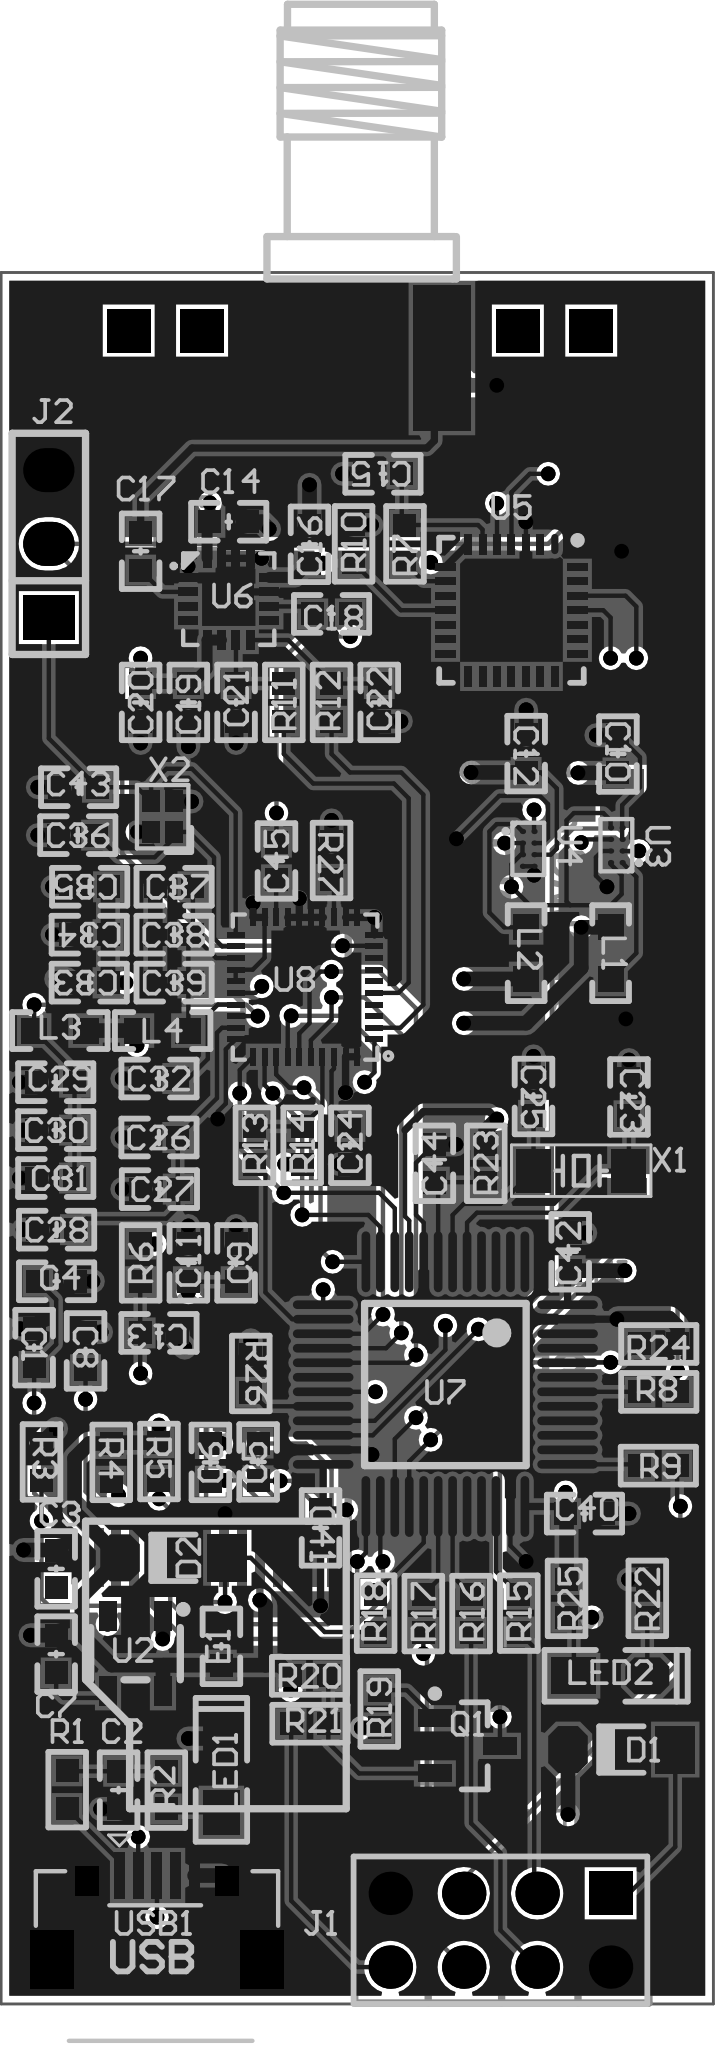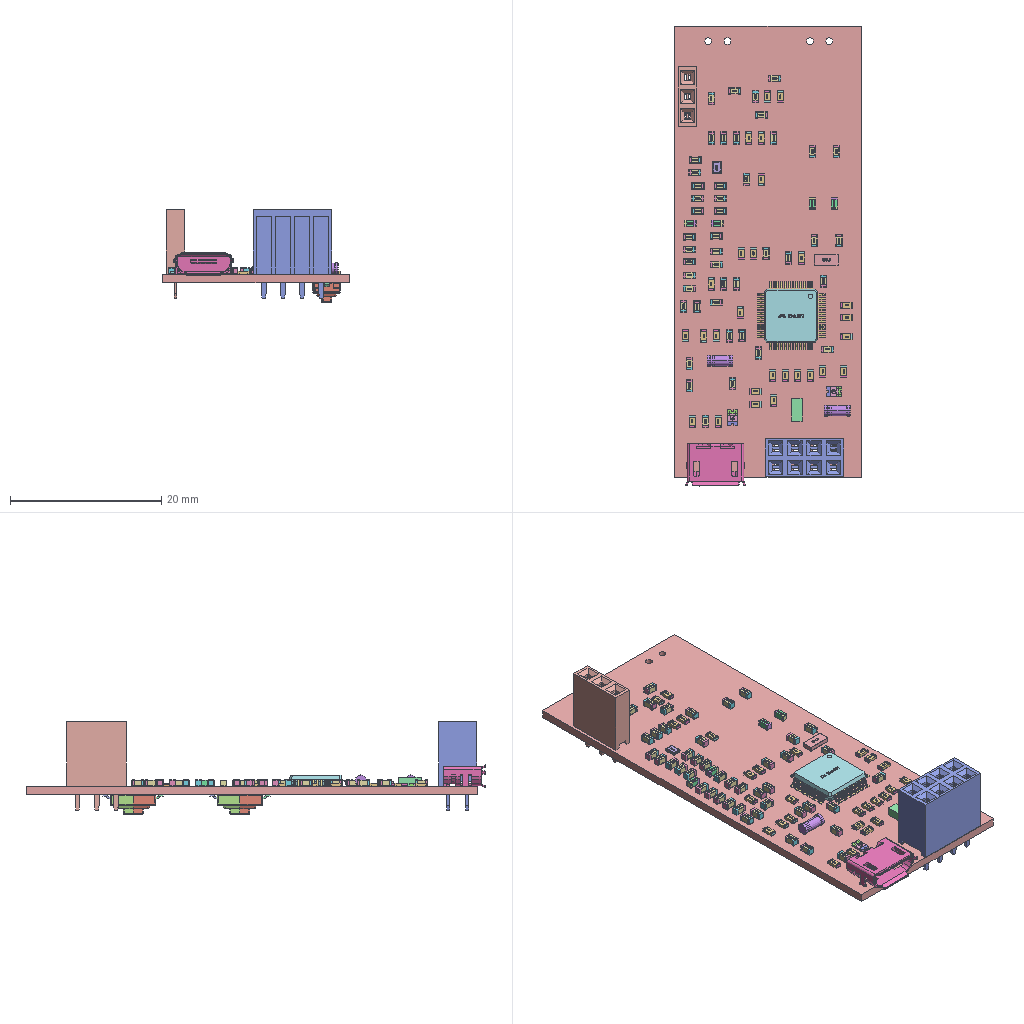Circuit board layout | Altium Designer | box 24.6 x 60.8 x 12.2 mm
Layer stack:
# Altium Designer layer stack of  (unit mm; dielectric type: 0 none, 1 core, 2 prepreg, 3 surface material)
index,name,kind,layer,copper_thickness_mm,dielectric_type,dielectric_thickness_mm,dielectric_material,dielectric_constant
0,Top Paste,other,,,,,,
1,Top Overlay,other,,,,,,
2,Top Solder,dielectric,,,3,0.0102,Solder Resist,3.5
3,Top Layer,copper,Top Layer,0.0356,,,,
4,Dielectric1,dielectric,,,1,0.32,FR-4,4.8
5,SIGN,copper,SIGN,0.0356,,,,
6,Dielectric3,dielectric,,,1,0.32,FR-4,4.8
7,VCC,copper,VCC,0.0356,,,,
8,Dielectric2,dielectric,,,2,0.32,FR-4,4.8
9,Bottom Layer,copper,Bottom Layer,0.0356,,,,
10,Bottom Solder,dielectric,,,3,0.0102,Solder Resist,3.5
11,Bottom Overlay,other,,,,,,
12,Bottom Paste,other,,,,,,
# drill layer pairs: low layer,high layer
drill_pair,Top Layer,Bottom Layer
Part placement:
Designator,Comment,Layer,Footprint,Center-X(mm),Center-Y(mm),Rotation
U1,0.91-OLED,BottomLayer,OLED0.91,4.987,15.367,270
X2,38.4MHZ,TopLayer,OSC_1612-4P,3.175,40.894,90
X1,16MHz,TopLayer,OSC_3215-2P,17.653,28.702,360
USB1,USB-5P,TopLayer,USB-MICRO_A,2.979,2.974,0
U8,DW3210,TopLayer,DW3210,8.101,35.025,180
U7,STM32F103C8T6,TopLayer,LQFP48_7X7,12.954,21.349,180
U6,SW8112Q,TopLayer,QFN-16_L3.0-W3.0-P0.50-BL-EP1.7,5.461,48.387,270
U5,CP2102,TopLayer,CP2102,15.24,48.006,270
U4,TPS62743YFPR,TopLayer,DSBGA-8_L1.6-W0.9-R2-C4-P0.40-BL,15.821,39.786,270
U3,TPS62743YFPR,TopLayer,DSBGA-8_L1.6-W0.9-R2-C4-P0.40-BL,18.869,39.913,90
U2,TPS736,TopLayer,SOT-23-5_L3.0-W1.7-P0.95-LS2.8-BR,2.236,12.065,90
SW2,3x6x5,BottomLayer,TSW_SMD-3*6*2.5,19.06,45.495,270
SW1,3x6x5,BottomLayer,TSW_SMD-3*6*2.5,19.187,31.398,270
R27,49R9,TopLayer,R_0603_L,9.017,39.385,270
R26,10K,TopLayer,R_0603_L,6.223,21.717,90
R25,10K,TopLayer,R_0603_L,17.145,13.97,90
R24,10K,TopLayer,R_0603_L,20.335,22.733,360
R23,1K,TopLayer,R_0603_L,14.351,28.956,90
R22,470R,TopLayer,R_0603_L,19.939,13.97,90
R21,1K,TopLayer,R_0603_L,8.27,9.652,360
R20,1K,TopLayer,R_0603_L,8.255,11.303,360
R19,1K,TopLayer,R_0603_L,10.668,10.16,90
R18,22R,TopLayer,R_0603_L,10.541,13.462,90
R17,22R,TopLayer,R_0603_L,12.192,13.447,90
R16,22R,TopLayer,R_0603_L,13.843,13.447,90
R15,22R,TopLayer,R_0603_L,15.494,13.462,90
R14,DNF,TopLayer,R_0603_L,8.001,29.576,90
R13,100R,TopLayer,R_0603_L,6.35,29.576,90
R12,0R,TopLayer,R_0603_L,9.017,44.831,90
R11,0R,TopLayer,R_0603_L,7.366,44.831,90
R10,10K,TopLayer,R_0603_L,9.779,50.292,270
R9,22R,TopLayer,R_0603_L,20.32,18.542,0
R8,0R,TopLayer,R_0603_L,20.335,21.082,0
R7,4.7K,TopLayer,R_0603_L,11.557,50.292,90
R6,4.7K,TopLayer,R_0603_L,2.413,25.527,90
R5,4.7K,TopLayer,R_0603_L,3.048,18.684,270
R4,4.7K,TopLayer,R_0603_L,1.397,18.654,270
R3,4.7K,TopLayer,R_0603_L,-1.016,18.669,270
R2,470R,TopLayer,R_0603_L,3.302,7.366,90
R1,B5R,TopLayer,R_0603_L,-0.127,7.381,90
Q1,S9012,TopLayer,SOT-23B_N,13.716,8.89,360
LED2,Red,TopLayer,LED_0805G,18.669,11.303,360
LED1,Red,TopLayer,LED_0805G,5.207,7.874,90
L4,600R,TopLayer,L_0603,3.175,33.528,180
L3,600R,TopLayer,L_0603,-0.381,33.528,360
L2,Inductor Iron,TopLayer,L_0603,15.748,36.195,270
L1,Inductor Iron,TopLayer,L_0603,18.669,36.195,90
J2,Female HDR1X3,TopLayer,Fe-HDR1X3/2.54-S,-0.762,50.292,180
J1,Female HDR2X4,TopLayer,Fe-HDR2X4/2.54-S,14.859,2.54,180
E1,22uF/6.3V,TopLayer,C_0603_L,5.207,12.319,90
D2,1N4148,TopLayer,MINI_MELF_(LL34),3.556,15.367,180
D1,SS34,TopLayer,MINI_MELF_(LL34),19.05,8.763,180
C45,2pF,TopLayer,C_0603_L,7.112,39.37,90
C44,100nF,TopLayer,C_0603_L,12.573,28.956,90
C43,8pF,TopLayer,C_0603_L,0.269,41.91,360
C42,100nF,TopLayer,C_0603_L,17.272,25.908,90
C41,100nF,TopLayer,C_0603_L,8.636,16.398,270
C40,100nF,TopLayer,C_0603_L,17.765,16.891,360
C39,10uF,TopLayer,C_0603_L,3.571,35.179,360
C38,100nF,TopLayer,C_0603_L,3.571,36.83,360
C37,4.7nF,TopLayer,C_0603_L,3.571,38.481,360
C36,8pF,TopLayer,C_0603_L,0.239,40.259,360
C35,10uF,TopLayer,C_0603_L,0.65,38.481,180
C34,100nF,TopLayer,C_0603_L,0.6351,36.83,180
C33,4.7nF,TopLayer,C_0603_L,0.6351,35.179,180
C32,220nF,TopLayer,C_0603_L,3.048,31.877,180
C31,10uF,TopLayer,C_0603_L,-0.523,28.448,360
C30,100nF,TopLayer,C_0603_L,-0.523,30.099,360
C29,4.7nF,TopLayer,C_0603_L,-0.523,31.75,360
C28,22uF,TopLayer,C_0603_L,-0.493,26.67,360
C27,100nF,TopLayer,C_0603_L,3.063,28.067,360
C26,2pF,TopLayer,C_0603_L,3.048,29.845,360
C25,20pF,TopLayer,C_0603_L,16.002,31.257,270
C24,100nF,TopLayer,C_0603_L,9.652,29.576,90
C23,20pF,TopLayer,C_0603_L,19.304,31.242,270
C22,1nF,TopLayer,C_0603_L,10.668,44.831,270
C21,1nF,TopLayer,C_0603_L,5.715,44.831,270
C20,1nF,TopLayer,C_0603_L,2.413,44.831,270
C19,1nF,TopLayer,C_0603_L,4.064,44.831,270
C18,100pF,TopLayer,C_0603_L,9.017,47.879,180
C17,100pF,TopLayer,C_0603_L,2.413,50.038,90
C16,1nF,TopLayer,C_0603_L,8.255,50.277,90
C15,4.7uF,TopLayer,C_0603_L,10.795,52.705,360
C14,1nF,TopLayer,C_0603_L,5.461,51.054,360
C13,4.7uF,TopLayer,C_0603_L,3.048,23.114,180
C12,10uF,TopLayer,C_0603_L,15.748,43.068,270
C11,4.7uF,TopLayer,C_0603_L,4.064,25.527,90
C10,10uF,TopLayer,C_0603_L,18.923,43.053,270
C9,100nF,TopLayer,C_0603_L,5.715,25.527,90
C8,2.2uF,TopLayer,C_0603_L,0.508,22.494,270
C7,100nF,TopLayer,C_0603_L,-0.508,12.05,270
C6,1uF,TopLayer,C_0603_L,4.826,18.654,90
C5,1uF,TopLayer,C_0603_L,6.477,18.669,90
C4,4.7uF,TopLayer,C_0603_L,-0.493,24.892,180
C3,10uF,TopLayer,C_0603_L,-0.5081,14.986,270
C2,100nF,TopLayer,C_0603_L,1.651,7.366,90
C1,100nF,TopLayer,C_0603_L,-1.27,22.606,270
ANT1,Partron,TopLayer,天线座5p,10.033,56.685,90
Pad and via stacks:
# Altium Designer via and pad stacks of  (unit mm). Each distinct definition once, with the count of objects using it.
# via: kind,start_layer,end_layer,hole_mm,diameter_mm,mode(0 simple;1 top-mid-bottom;2 full stack),diameter_per_layer,count,example_net
# pad: kind,layer,hole_mm,hole_type(0 round;1 square;2 slot),plating,top_size,top_shape(1 round;2 rect;3 octagon;9 rounded rect),mid_size,bottom_size,mode,footprint,size_per_layer,count,example
pad,Multi-Layer,0.5,2,plated,1.5x2,2,1.5x2,1.5x2,0,USB-MICRO_A,,2,USB1.5
pad,Multi-Layer,0.5,0,plated,0.8x1,2,0.8x1,0.8x1,0,USB-MICRO_A,,2,USB1.5
pad,Multi-Layer,0.9,0,plated,1.5x1.5,2,1.5x1.5,1.5x1.5,0,Fe-HDR2X4/2.54-S,,1,J1.1
pad,Multi-Layer,0.9,0,plated,1.5x1.5,1,1.5x1.5,1.5x1.5,0,Fe-HDR2X4/2.54-S,,7,J1.2
pad,Multi-Layer,0.8128,0,plated,1.524x1.778,2,1.524x1.778,1.524x1.778,0,Fe-HDR1X3/2.54-S,,1,J2.1
pad,Multi-Layer,0.8128,0,plated,1.524x1.778,1,1.524x1.778,1.524x1.778,0,Fe-HDR1X3/2.54-S,,2,J2.2
pad,Multi-Layer,0.9,0,plated,1.5x1.5,2,1.5x1.5,1.5x1.5,0,,,4,0
pad,Top Layer,0,0,plated,0.889x0.889,2,0.889x0.889,0.889x0.889,0,L 0603,,8,L2.1
pad,Top Layer,0,0,plated,1.2x1.5,2,1.2x1.5,1.2x1.5,0,OSC 3215-2P,,2,X1.1
pad,Top Layer,0,0,plated,0.762x0.762,2,0.762x0.762,0.762x0.762,0,C 0603_L,,92,E1.1
pad,Top Layer,0,0,plated,1.6x0.35,2,1.6x0.35,1.6x0.35,0,USB-MICRO_A,,5,USB1.2
pad,Top Layer,0,0,plated,1.62x1.37,3,1.62x1.37,1.62x1.37,0,MINI_MELF (LL34),,2,D1.2
pad,Top Layer,0,0,plated,1.62x1.37,2,1.62x1.37,1.62x1.37,0,MINI_MELF (LL34),,2,D1.1
pad,Top Layer,0,0,plated,1x0.6,2,1x0.6,1x0.6,0,SOT-23-5_L3.0-W1.7-P0.95-LS2.8-BR,,5,U2.1
pad,Top Layer,0,0,plated,0.762x0.762,2,0.762x0.762,0.762x0.762,0,R 0603_L,,54,R1.2
pad,Top Layer,0,0,plated,0.184x0.184,1,0.184x0.184,0.184x0.184,0,DSBGA-8_L1.6-W0.9-R2-C4-P0.40-BL,,16,U3.D2
pad,Top Layer,0,0,plated,1.524x1.27,2,1.524x1.27,1.524x1.27,0,LED 0805G,,2,LED1.1
pad,Top Layer,0,0,plated,1.524x1.27,3,1.524x1.27,1.524x1.27,0,LED 0805G,,2,LED1.2
pad,Top Layer,0,0,plated,0.25x0.7,1,0.25x0.7,0.25x0.7,0,CP2102,,1,U5.1
pad,Top Layer,0,0,plated,0.25x0.7,2,0.25x0.7,0.25x0.7,0,CP2102,,27,U5.2
pad,Top Layer,0,0,plated,3.15x3.15,2,3.15x3.15,3.15x3.15,0,CP2102,,1,U5.29
pad,Top Layer,0,0,plated,0.28x0.665,2,0.28x0.665,0.28x0.665,0,QFN-16_L3.0-W3.0-P0.50-BL-EP1.7,,8,U6.1
pad,Top Layer,0,0,plated,0.665x0.28,2,0.665x0.28,0.665x0.28,0,QFN-16_L3.0-W3.0-P0.50-BL-EP1.7,,8,U6.5
pad,Top Layer,0,0,plated,1.75x1.75,2,1.75x1.75,1.75x1.75,0,QFN-16_L3.0-W3.0-P0.50-BL-EP1.7,,1,U6.17
pad,Top Layer,0,0,plated,0.3x2.1,1,0.3x2.1,0.3x2.1,0,LQFP48 7X7,,48,U7.48
pad,Top Layer,0,0,plated,0.6x0.2,2,0.6x0.2,0.6x0.2,0,DW3210,,40,U8.1
pad,Top Layer,0,0,plated,0.6x1.15,2,0.6x1.15,0.6x1.15,0,SOT-23B_N,,3,Q1.1
pad,Top Layer,0,0,plated,0.6x0.75,2,0.6x0.75,0.6x0.75,0,OSC 1612-4P,,4,X2.1
pad,Top Layer,0,0,plated,5x1.3,2,5x1.3,5x1.3,0,\u00CC\u00EC\u00CF\u00DF\u00D7\u00F95p,,1,ANT1.5
pad,Top Layer,0,0,plated,5x2,2,5x2,5x2,0,\u00CC\u00EC\u00CF\u00DF\u00D7\u00F95p,,2,ANT1.2
pad,Bottom Layer,0,0,plated,2x1.5,2,2x1.5,2x1.5,0,TSW SMD-3*6*2.5,,4,SW2.1
pad,Bottom Layer,0,0,plated,2x0.32,2,2x0.32,2x0.32,0,OLED0.91,,14,U1.1
pad,Bottom Layer,0,0,plated,5x2,2,5x2,5x2,0,\u00CC\u00EC\u00CF\u00DF\u00D7\u00F95p,,2,ANT1.4
via,Top Layer,Bottom Layer,0.254,0.508,0,,149,3V3
via,Top Layer,Bottom Layer,0.33,0.66,0,,4,GND
Copper pours:
name,layer,net,type(0 solid;1 hatched;2 none)
D,SIGN,GND,0
D,VCC,3V3,0
D,Top Layer,GND,0
D,Bottom Layer,GND,0
Design rules, without the lines most boards share:
# Altium Designer design rules of  (exported by Altium Designer, unit mm)
# columns: name | kind | enabled | priority | scope1 | scope2 | descriptor | typed fields (field=value)
SilkToSilkClearance | 55 | enabled | 1 | All | All | Silk to Silk (Clearance=0mil) (All),(All) |
SilkscreenOverComponentPads | 54 | enabled | 1 | IsPad | All | Silk To Solder Mask (Clearance=0mil) (IsPad),(All) |
MinimumSolderMaskSliver | 53 | enabled | 1 | All | All | Minimum Solder Mask Sliver (Gap=0mil) (All),(All) |
HoleToHoleClearance | 52 | enabled | 1 | All | All | Hole To Hole Clearance (Gap=10mil) (All),(All) | gap=0.254
DiffPairsRouting | 51 | enabled | 1 | All | All | Differential Pairs Uncoupled Length using the Gap Constraints (Min=10mil) (Max=10mil) (Prefered=10mil)  and Width Constraints (Min=15mil) (Max=15mil) (Prefered=15mil) (All) |
SolderMaskExpansion | 13 | enabled | 1 | All | All | Solder Mask Expansion (Expansion =4mil) (All) | expansion=0.1016
PasteMaskExpansion | 14 | enabled | 1 | All | All | Paste Mask Expansion (Expansion =0mil) (All) | expansion=0
RoutingVias | 11 | enabled | 1 | All | All | Routing Via (MinHoleWidth=11.811mil) (MaxHoleWidth=11.811mil) (PreferredHoleWidth=11.811mil) (MinWidth=17.716mil) (MaxWidth=17.716mil) (PreferedWidth=17.716mil) (All) | via_min_hole=0.3 via_max_hole=0.3 via_preferred_diameter=0.45 via_preferred_hole=0.3
Width | 2 | enabled | 1 | All | All | Width Constraint (Min=5mil) (Max=20mil) (Preferred=5mil) (All) |
PolygonConnect | 20 | enabled | 1 | All | All | Polygon Connect Rule(Direct Connect )(Conductor Width=10mil) (Relief Angle=90 Angle) (Entries=4) (Air Gap Width=10mil) (All),(All) | connect_style(0=relief,1=direct,2=none)=1 relief_conductor_width=0.254 relief_entries=4
PlaneConnect | 6 | enabled | 1 | All | All | Power Plane Connect Rule(Direct Connect )(Expansion=20mil) (Conductor Width=10mil) (Air Gap=10mil) (Entries=4) (All) | relief_conductor_width=0.254 relief_entries=4 relief_expansion=0.508
Clearance | 0 | enabled | 1 | All | All | Clearance Constraint (Gap=6mil) (All),(All) | gap=0.1524
Classes set for this board:
# Altium Designer classes of  (member kind: 0 net, 1 component, 2 from-to, 3 pad, 4 layer, 5 differential pair, 6 design channel, 7 polygon, 8 structure, 9 xSignal)
# columns: class name | member kind | superclass | members
Sheet1 | 1 | no | ANT1; C1; C2; C3; C4; C5; C6; C7; C8; C9; C10; C11; C12; C13; C14; C15; C16; C17; C18; C19; C20; C21; C22; C23; C24; C25; C26; C27; C28; C29; C30; C31; C32; C33; C34; C35; C36; C37; C38; C39; C40; C41; C42; C43; C44; C45; D1; D2; E1; J1; J2; L1; L2; L3; L4; LED1; LED2; Q1; R1; R2; R3; R4; R5; R6; R7; R8; R9; R10; R11; R12; R13; R14; R15; R16; R17; R18; R19; R20; R21; R22; R23; R24; R25; R26; R27; SW1; SW2; U2; U3; U4; U5; U6; U7; U8; USB1; X1; X2; U1;